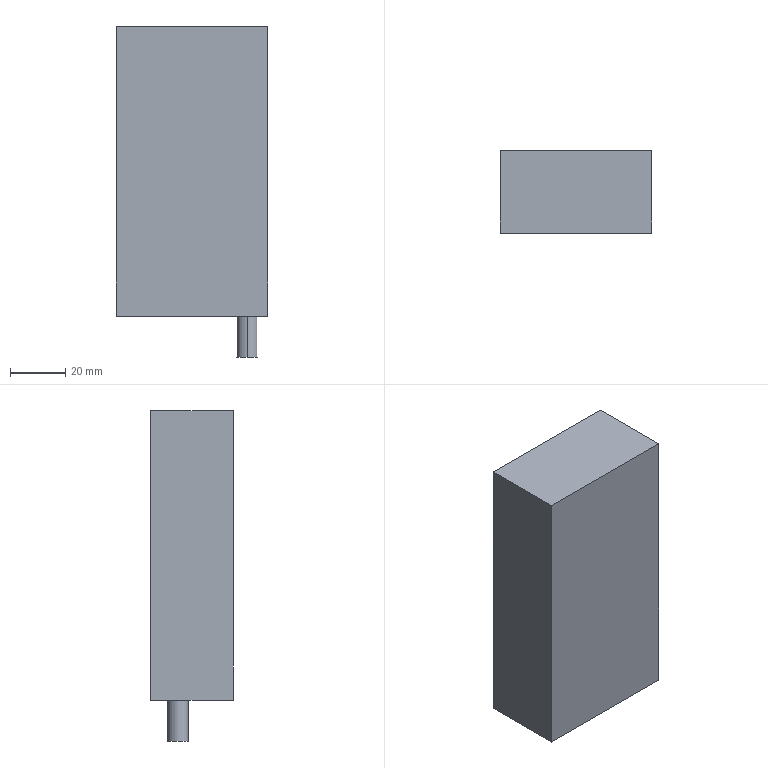Part | SolidWorks | features BaseBody 1 | 1 solid | 33 faces | box 55 x 30 x 120 mm | volume 172847 mm3 | cylinder 14 | cone 12 | plane 7 | commonest cylinder face diameters 4.2 x12 7.5 x2
STEP:
#1=CARTESIAN_POINT('',(47.5,23.75,-15.));
#2=VERTEX_POINT('',#1);
#3=CARTESIAN_POINT('',(47.5,16.25,-15.));
#4=VERTEX_POINT('',#3);
#5=CARTESIAN_POINT('',(47.5,20.,-15.));
#6=DIRECTION('',(0.,0.,-1.));
#7=DIRECTION('',(0.,-1.,0.));
#8=AXIS2_PLACEMENT_3D('',#5,#6,#7);
#9=CIRCLE('',#8,3.75);
#10=EDGE_CURVE('',#2,#4,#9,.T.);
#11=ORIENTED_EDGE('',*,*,#10,.F.);
#12=CARTESIAN_POINT('',(47.5,23.75,0.));
#13=VERTEX_POINT('',#12);
#14=CARTESIAN_POINT('',(47.5,23.75,-15.));
#15=DIRECTION('',(0.,0.,1.));
#16=VECTOR('',#15,1000.);
#17=LINE('',#14,#16);
#18=EDGE_CURVE('',#2,#13,#17,.T.);
#19=ORIENTED_EDGE('',*,*,#18,.T.);
#20=CARTESIAN_POINT('',(47.5,16.25,0.));
#21=VERTEX_POINT('',#20);
#22=CARTESIAN_POINT('',(47.5,20.,0.));
#23=DIRECTION('',(0.,0.,1.));
#24=DIRECTION('',(0.,-1.,0.));
#25=AXIS2_PLACEMENT_3D('',#22,#23,#24);
#26=CIRCLE('',#25,3.75);
#27=EDGE_CURVE('',#21,#13,#26,.T.);
#28=ORIENTED_EDGE('',*,*,#27,.F.);
#29=CARTESIAN_POINT('',(47.5,16.25,-15.));
#30=DIRECTION('',(0.,0.,1.));
#31=VECTOR('',#30,1000.);
#32=LINE('',#29,#31);
#33=EDGE_CURVE('',#4,#21,#32,.T.);
#34=ORIENTED_EDGE('',*,*,#33,.F.);
#35=EDGE_LOOP('',(#11,#19,#28,#34));
#36=FACE_OUTER_BOUND('',#35,.T.);
#37=CARTESIAN_POINT('',(47.5,20.,-15.));
#38=DIRECTION('',(0.,0.,1.));
#39=DIRECTION('',(0.,-1.,0.));
#40=AXIS2_PLACEMENT_3D('',#37,#38,#39);
#41=CYLINDRICAL_SURFACE('',#40,3.75);
#42=ADVANCED_FACE('',(#36),#41,.T.);
#43=CARTESIAN_POINT('',(50.,17.6,17.1));
#44=VERTEX_POINT('',#43);
#45=CARTESIAN_POINT('',(50.,17.6,12.9));
#46=VERTEX_POINT('',#45);
#47=CARTESIAN_POINT('',(50.,17.6,15.));
#48=DIRECTION('',(0.,-1.,0.));
#49=DIRECTION('',(0.,0.,1.));
#50=AXIS2_PLACEMENT_3D('',#47,#48,#49);
#51=CIRCLE('',#50,2.1);
#52=EDGE_CURVE('',#44,#46,#51,.T.);
#53=ORIENTED_EDGE('',*,*,#52,.T.);
#54=CARTESIAN_POINT('',(50.,30.,12.9));
#55=VERTEX_POINT('',#54);
#56=CARTESIAN_POINT('',(50.,17.6,12.9));
#57=DIRECTION('',(0.,1.,0.));
#58=VECTOR('',#57,1000.);
#59=LINE('',#56,#58);
#60=EDGE_CURVE('',#46,#55,#59,.T.);
#61=ORIENTED_EDGE('',*,*,#60,.T.);
#62=CARTESIAN_POINT('',(50.,30.,17.1));
#63=VERTEX_POINT('',#62);
#64=CARTESIAN_POINT('',(50.,30.,15.));
#65=DIRECTION('',(0.,1.,0.));
#66=DIRECTION('',(0.,0.,1.));
#67=AXIS2_PLACEMENT_3D('',#64,#65,#66);
#68=CIRCLE('',#67,2.1);
#69=EDGE_CURVE('',#55,#63,#68,.T.);
#70=ORIENTED_EDGE('',*,*,#69,.T.);
#71=CARTESIAN_POINT('',(50.,17.6,17.1));
#72=DIRECTION('',(0.,1.,0.));
#73=VECTOR('',#72,1000.);
#74=LINE('',#71,#73);
#75=EDGE_CURVE('',#44,#63,#74,.T.);
#76=ORIENTED_EDGE('',*,*,#75,.F.);
#77=EDGE_LOOP('',(#53,#61,#70,#76));
#78=FACE_OUTER_BOUND('',#77,.T.);
#79=CARTESIAN_POINT('',(50.,17.6,15.));
#80=DIRECTION('',(0.,1.,0.));
#81=DIRECTION('',(0.,0.,1.));
#82=AXIS2_PLACEMENT_3D('',#79,#80,#81);
#83=CYLINDRICAL_SURFACE('',#82,2.1);
#84=ADVANCED_FACE('',(#78),#83,.F.);
#85=CARTESIAN_POINT('',(5.,17.6,17.1));
#86=VERTEX_POINT('',#85);
#87=CARTESIAN_POINT('',(5.,17.6,12.9));
#88=VERTEX_POINT('',#87);
#89=CARTESIAN_POINT('',(5.,17.6,15.));
#90=DIRECTION('',(0.,-1.,0.));
#91=DIRECTION('',(0.,0.,1.));
#92=AXIS2_PLACEMENT_3D('',#89,#90,#91);
#93=CIRCLE('',#92,2.1);
#94=EDGE_CURVE('',#86,#88,#93,.T.);
#95=ORIENTED_EDGE('',*,*,#94,.T.);
#96=CARTESIAN_POINT('',(5.,30.,12.9));
#97=VERTEX_POINT('',#96);
#98=CARTESIAN_POINT('',(5.,17.6,12.9));
#99=DIRECTION('',(0.,1.,0.));
#100=VECTOR('',#99,1000.);
#101=LINE('',#98,#100);
#102=EDGE_CURVE('',#88,#97,#101,.T.);
#103=ORIENTED_EDGE('',*,*,#102,.T.);
#104=CARTESIAN_POINT('',(5.,30.,17.1));
#105=VERTEX_POINT('',#104);
#106=CARTESIAN_POINT('',(5.,30.,15.));
#107=DIRECTION('',(0.,1.,0.));
#108=DIRECTION('',(0.,0.,1.));
#109=AXIS2_PLACEMENT_3D('',#106,#107,#108);
#110=CIRCLE('',#109,2.1);
#111=EDGE_CURVE('',#97,#105,#110,.T.);
#112=ORIENTED_EDGE('',*,*,#111,.T.);
#113=CARTESIAN_POINT('',(5.,17.6,17.1));
#114=DIRECTION('',(0.,1.,0.));
#115=VECTOR('',#114,1000.);
#116=LINE('',#113,#115);
#117=EDGE_CURVE('',#86,#105,#116,.T.);
#118=ORIENTED_EDGE('',*,*,#117,.F.);
#119=EDGE_LOOP('',(#95,#103,#112,#118));
#120=FACE_OUTER_BOUND('',#119,.T.);
#121=CARTESIAN_POINT('',(5.,17.6,15.));
#122=DIRECTION('',(0.,1.,0.));
#123=DIRECTION('',(0.,0.,1.));
#124=AXIS2_PLACEMENT_3D('',#121,#122,#123);
#125=CYLINDRICAL_SURFACE('',#124,2.1);
#126=ADVANCED_FACE('',(#120),#125,.F.);
#127=CARTESIAN_POINT('',(50.,17.6,54.6));
#128=VERTEX_POINT('',#127);
#129=CARTESIAN_POINT('',(50.,17.6,50.4));
#130=VERTEX_POINT('',#129);
#131=CARTESIAN_POINT('',(50.,17.6,52.5));
#132=DIRECTION('',(0.,-1.,0.));
#133=DIRECTION('',(0.,0.,1.));
#134=AXIS2_PLACEMENT_3D('',#131,#132,#133);
#135=CIRCLE('',#134,2.1);
#136=EDGE_CURVE('',#128,#130,#135,.T.);
#137=ORIENTED_EDGE('',*,*,#136,.T.);
#138=CARTESIAN_POINT('',(50.,30.,50.4));
#139=VERTEX_POINT('',#138);
#140=CARTESIAN_POINT('',(50.,17.6,50.4));
#141=DIRECTION('',(0.,1.,0.));
#142=VECTOR('',#141,1000.);
#143=LINE('',#140,#142);
#144=EDGE_CURVE('',#130,#139,#143,.T.);
#145=ORIENTED_EDGE('',*,*,#144,.T.);
#146=CARTESIAN_POINT('',(50.,30.,54.6));
#147=VERTEX_POINT('',#146);
#148=CARTESIAN_POINT('',(50.,30.,52.5));
#149=DIRECTION('',(0.,1.,0.));
#150=DIRECTION('',(0.,0.,1.));
#151=AXIS2_PLACEMENT_3D('',#148,#149,#150);
#152=CIRCLE('',#151,2.1);
#153=EDGE_CURVE('',#139,#147,#152,.T.);
#154=ORIENTED_EDGE('',*,*,#153,.T.);
#155=CARTESIAN_POINT('',(50.,17.6,54.6));
#156=DIRECTION('',(0.,1.,0.));
#157=VECTOR('',#156,1000.);
#158=LINE('',#155,#157);
#159=EDGE_CURVE('',#128,#147,#158,.T.);
#160=ORIENTED_EDGE('',*,*,#159,.F.);
#161=EDGE_LOOP('',(#137,#145,#154,#160));
#162=FACE_OUTER_BOUND('',#161,.T.);
#163=CARTESIAN_POINT('',(50.,17.6,52.5));
#164=DIRECTION('',(0.,1.,0.));
#165=DIRECTION('',(0.,0.,1.));
#166=AXIS2_PLACEMENT_3D('',#163,#164,#165);
#167=CYLINDRICAL_SURFACE('',#166,2.1);
#168=ADVANCED_FACE('',(#162),#167,.F.);
#169=CARTESIAN_POINT('',(5.,17.6,54.6));
#170=VERTEX_POINT('',#169);
#171=CARTESIAN_POINT('',(5.,17.6,50.4));
#172=VERTEX_POINT('',#171);
#173=CARTESIAN_POINT('',(5.,17.6,52.5));
#174=DIRECTION('',(0.,-1.,0.));
#175=DIRECTION('',(0.,0.,1.));
#176=AXIS2_PLACEMENT_3D('',#173,#174,#175);
#177=CIRCLE('',#176,2.1);
#178=EDGE_CURVE('',#170,#172,#177,.T.);
#179=ORIENTED_EDGE('',*,*,#178,.T.);
#180=CARTESIAN_POINT('',(5.,30.,50.4));
#181=VERTEX_POINT('',#180);
#182=CARTESIAN_POINT('',(5.,17.6,50.4));
#183=DIRECTION('',(0.,1.,0.));
#184=VECTOR('',#183,1000.);
#185=LINE('',#182,#184);
#186=EDGE_CURVE('',#172,#181,#185,.T.);
#187=ORIENTED_EDGE('',*,*,#186,.T.);
#188=CARTESIAN_POINT('',(5.,30.,54.6));
#189=VERTEX_POINT('',#188);
#190=CARTESIAN_POINT('',(5.,30.,52.5));
#191=DIRECTION('',(0.,1.,0.));
#192=DIRECTION('',(0.,0.,1.));
#193=AXIS2_PLACEMENT_3D('',#190,#191,#192);
#194=CIRCLE('',#193,2.1);
#195=EDGE_CURVE('',#181,#189,#194,.T.);
#196=ORIENTED_EDGE('',*,*,#195,.T.);
#197=CARTESIAN_POINT('',(5.,17.6,54.6));
#198=DIRECTION('',(0.,1.,0.));
#199=VECTOR('',#198,1000.);
#200=LINE('',#197,#199);
#201=EDGE_CURVE('',#170,#189,#200,.T.);
#202=ORIENTED_EDGE('',*,*,#201,.F.);
#203=EDGE_LOOP('',(#179,#187,#196,#202));
#204=FACE_OUTER_BOUND('',#203,.T.);
#205=CARTESIAN_POINT('',(5.,17.6,52.5));
#206=DIRECTION('',(0.,1.,0.));
#207=DIRECTION('',(0.,0.,1.));
#208=AXIS2_PLACEMENT_3D('',#205,#206,#207);
#209=CYLINDRICAL_SURFACE('',#208,2.1);
#210=ADVANCED_FACE('',(#204),#209,.F.);
#211=CARTESIAN_POINT('',(50.,17.6,92.1));
#212=VERTEX_POINT('',#211);
#213=CARTESIAN_POINT('',(50.,17.6,87.9));
#214=VERTEX_POINT('',#213);
#215=CARTESIAN_POINT('',(50.,17.6,90.));
#216=DIRECTION('',(0.,-1.,0.));
#217=DIRECTION('',(0.,0.,1.));
#218=AXIS2_PLACEMENT_3D('',#215,#216,#217);
#219=CIRCLE('',#218,2.1);
#220=EDGE_CURVE('',#212,#214,#219,.T.);
#221=ORIENTED_EDGE('',*,*,#220,.T.);
#222=CARTESIAN_POINT('',(50.,30.,87.9));
#223=VERTEX_POINT('',#222);
#224=CARTESIAN_POINT('',(50.,17.6,87.9));
#225=DIRECTION('',(0.,1.,0.));
#226=VECTOR('',#225,1000.);
#227=LINE('',#224,#226);
#228=EDGE_CURVE('',#214,#223,#227,.T.);
#229=ORIENTED_EDGE('',*,*,#228,.T.);
#230=CARTESIAN_POINT('',(50.,30.,92.1));
#231=VERTEX_POINT('',#230);
#232=CARTESIAN_POINT('',(50.,30.,90.));
#233=DIRECTION('',(0.,1.,0.));
#234=DIRECTION('',(0.,0.,1.));
#235=AXIS2_PLACEMENT_3D('',#232,#233,#234);
#236=CIRCLE('',#235,2.1);
#237=EDGE_CURVE('',#223,#231,#236,.T.);
#238=ORIENTED_EDGE('',*,*,#237,.T.);
#239=CARTESIAN_POINT('',(50.,17.6,92.1));
#240=DIRECTION('',(0.,1.,0.));
#241=VECTOR('',#240,1000.);
#242=LINE('',#239,#241);
#243=EDGE_CURVE('',#212,#231,#242,.T.);
#244=ORIENTED_EDGE('',*,*,#243,.F.);
#245=EDGE_LOOP('',(#221,#229,#238,#244));
#246=FACE_OUTER_BOUND('',#245,.T.);
#247=CARTESIAN_POINT('',(50.,17.6,90.));
#248=DIRECTION('',(0.,1.,0.));
#249=DIRECTION('',(0.,0.,1.));
#250=AXIS2_PLACEMENT_3D('',#247,#248,#249);
#251=CYLINDRICAL_SURFACE('',#250,2.1);
#252=ADVANCED_FACE('',(#246),#251,.F.);
#253=CARTESIAN_POINT('',(5.,17.6,92.1));
#254=VERTEX_POINT('',#253);
#255=CARTESIAN_POINT('',(5.,17.6,87.9));
#256=VERTEX_POINT('',#255);
#257=CARTESIAN_POINT('',(5.,17.6,90.));
#258=DIRECTION('',(0.,-1.,0.));
#259=DIRECTION('',(0.,0.,1.));
#260=AXIS2_PLACEMENT_3D('',#257,#258,#259);
#261=CIRCLE('',#260,2.1);
#262=EDGE_CURVE('',#254,#256,#261,.T.);
#263=ORIENTED_EDGE('',*,*,#262,.T.);
#264=CARTESIAN_POINT('',(5.,30.,87.9));
#265=VERTEX_POINT('',#264);
#266=CARTESIAN_POINT('',(5.,17.6,87.9));
#267=DIRECTION('',(0.,1.,0.));
#268=VECTOR('',#267,1000.);
#269=LINE('',#266,#268);
#270=EDGE_CURVE('',#256,#265,#269,.T.);
#271=ORIENTED_EDGE('',*,*,#270,.T.);
#272=CARTESIAN_POINT('',(5.,30.,92.1));
#273=VERTEX_POINT('',#272);
#274=CARTESIAN_POINT('',(5.,30.,90.));
#275=DIRECTION('',(0.,1.,0.));
#276=DIRECTION('',(0.,0.,1.));
#277=AXIS2_PLACEMENT_3D('',#274,#275,#276);
#278=CIRCLE('',#277,2.1);
#279=EDGE_CURVE('',#265,#273,#278,.T.);
#280=ORIENTED_EDGE('',*,*,#279,.T.);
#281=CARTESIAN_POINT('',(5.,17.6,92.1));
#282=DIRECTION('',(0.,1.,0.));
#283=VECTOR('',#282,1000.);
#284=LINE('',#281,#283);
#285=EDGE_CURVE('',#254,#273,#284,.T.);
#286=ORIENTED_EDGE('',*,*,#285,.F.);
#287=EDGE_LOOP('',(#263,#271,#280,#286));
#288=FACE_OUTER_BOUND('',#287,.T.);
#289=CARTESIAN_POINT('',(5.,17.6,90.));
#290=DIRECTION('',(0.,1.,0.));
#291=DIRECTION('',(0.,0.,1.));
#292=AXIS2_PLACEMENT_3D('',#289,#290,#291);
#293=CYLINDRICAL_SURFACE('',#292,2.1);
#294=ADVANCED_FACE('',(#288),#293,.F.);
#295=CARTESIAN_POINT('',(50.,16.338,15.));
#296=VERTEX_POINT('',#295);
#297=CARTESIAN_POINT('',(50.,16.338,15.));
#298=DIRECTION('',(0.,0.515,0.8572));
#299=VECTOR('',#298,1000.);
#300=LINE('',#297,#299);
#301=EDGE_CURVE('',#296,#44,#300,.T.);
#302=ORIENTED_EDGE('',*,*,#301,.F.);
#303=CARTESIAN_POINT('',(50.,16.338,15.));
#304=DIRECTION('',(0.,0.515,-0.8572));
#305=VECTOR('',#304,1000.);
#306=LINE('',#303,#305);
#307=EDGE_CURVE('',#296,#46,#306,.T.);
#308=ORIENTED_EDGE('',*,*,#307,.T.);
#309=ORIENTED_EDGE('',*,*,#52,.F.);
#310=EDGE_LOOP('',(#302,#308,#309));
#311=FACE_OUTER_BOUND('',#310,.T.);
#312=CARTESIAN_POINT('',(50.,1016.338,15.));
#313=DIRECTION('',(0.,1.,0.));
#314=DIRECTION('',(0.,0.,1.));
#315=AXIS2_PLACEMENT_3D('',#312,#313,#314);
#316=CONICAL_SURFACE('',#315,1664.279,1.03);
#317=ADVANCED_FACE('',(#311),#316,.F.);
#318=CARTESIAN_POINT('',(5.,16.338,15.));
#319=VERTEX_POINT('',#318);
#320=CARTESIAN_POINT('',(5.,16.338,15.));
#321=DIRECTION('',(0.,0.515,0.8572));
#322=VECTOR('',#321,1000.);
#323=LINE('',#320,#322);
#324=EDGE_CURVE('',#319,#86,#323,.T.);
#325=ORIENTED_EDGE('',*,*,#324,.F.);
#326=CARTESIAN_POINT('',(5.,16.338,15.));
#327=DIRECTION('',(0.,0.515,-0.8572));
#328=VECTOR('',#327,1000.);
#329=LINE('',#326,#328);
#330=EDGE_CURVE('',#319,#88,#329,.T.);
#331=ORIENTED_EDGE('',*,*,#330,.T.);
#332=ORIENTED_EDGE('',*,*,#94,.F.);
#333=EDGE_LOOP('',(#325,#331,#332));
#334=FACE_OUTER_BOUND('',#333,.T.);
#335=CARTESIAN_POINT('',(5.,1016.338,15.));
#336=DIRECTION('',(0.,1.,0.));
#337=DIRECTION('',(0.,0.,1.));
#338=AXIS2_PLACEMENT_3D('',#335,#336,#337);
#339=CONICAL_SURFACE('',#338,1664.279,1.03);
#340=ADVANCED_FACE('',(#334),#339,.F.);
#341=CARTESIAN_POINT('',(50.,16.338,52.5));
#342=VERTEX_POINT('',#341);
#343=CARTESIAN_POINT('',(50.,16.338,52.5));
#344=DIRECTION('',(0.,0.515,0.8572));
#345=VECTOR('',#344,1000.);
#346=LINE('',#343,#345);
#347=EDGE_CURVE('',#342,#128,#346,.T.);
#348=ORIENTED_EDGE('',*,*,#347,.F.);
#349=CARTESIAN_POINT('',(50.,16.338,52.5));
#350=DIRECTION('',(0.,0.515,-0.8572));
#351=VECTOR('',#350,1000.);
#352=LINE('',#349,#351);
#353=EDGE_CURVE('',#342,#130,#352,.T.);
#354=ORIENTED_EDGE('',*,*,#353,.T.);
#355=ORIENTED_EDGE('',*,*,#136,.F.);
#356=EDGE_LOOP('',(#348,#354,#355));
#357=FACE_OUTER_BOUND('',#356,.T.);
#358=CARTESIAN_POINT('',(50.,1016.338,52.5));
#359=DIRECTION('',(0.,1.,0.));
#360=DIRECTION('',(0.,0.,1.));
#361=AXIS2_PLACEMENT_3D('',#358,#359,#360);
#362=CONICAL_SURFACE('',#361,1664.279,1.03);
#363=ADVANCED_FACE('',(#357),#362,.F.);
#364=CARTESIAN_POINT('',(5.,16.338,52.5));
#365=VERTEX_POINT('',#364);
#366=CARTESIAN_POINT('',(5.,16.338,52.5));
#367=DIRECTION('',(0.,0.515,0.8572));
#368=VECTOR('',#367,1000.);
#369=LINE('',#366,#368);
#370=EDGE_CURVE('',#365,#170,#369,.T.);
#371=ORIENTED_EDGE('',*,*,#370,.F.);
#372=CARTESIAN_POINT('',(5.,16.338,52.5));
#373=DIRECTION('',(0.,0.515,-0.8572));
#374=VECTOR('',#373,1000.);
#375=LINE('',#372,#374);
#376=EDGE_CURVE('',#365,#172,#375,.T.);
#377=ORIENTED_EDGE('',*,*,#376,.T.);
#378=ORIENTED_EDGE('',*,*,#178,.F.);
#379=EDGE_LOOP('',(#371,#377,#378));
#380=FACE_OUTER_BOUND('',#379,.T.);
#381=CARTESIAN_POINT('',(5.,1016.338,52.5));
#382=DIRECTION('',(0.,1.,0.));
#383=DIRECTION('',(0.,0.,1.));
#384=AXIS2_PLACEMENT_3D('',#381,#382,#383);
#385=CONICAL_SURFACE('',#384,1664.279,1.03);
#386=ADVANCED_FACE('',(#380),#385,.F.);
#387=CARTESIAN_POINT('',(50.,16.338,90.));
#388=VERTEX_POINT('',#387);
#389=CARTESIAN_POINT('',(50.,16.338,90.));
#390=DIRECTION('',(0.,0.515,0.8572));
#391=VECTOR('',#390,1000.);
#392=LINE('',#389,#391);
#393=EDGE_CURVE('',#388,#212,#392,.T.);
#394=ORIENTED_EDGE('',*,*,#393,.F.);
#395=CARTESIAN_POINT('',(50.,16.338,90.));
#396=DIRECTION('',(0.,0.515,-0.8572));
#397=VECTOR('',#396,1000.);
#398=LINE('',#395,#397);
#399=EDGE_CURVE('',#388,#214,#398,.T.);
#400=ORIENTED_EDGE('',*,*,#399,.T.);
#401=ORIENTED_EDGE('',*,*,#220,.F.);
#402=EDGE_LOOP('',(#394,#400,#401));
#403=FACE_OUTER_BOUND('',#402,.T.);
#404=CARTESIAN_POINT('',(50.,1016.338,90.));
#405=DIRECTION('',(0.,1.,0.));
#406=DIRECTION('',(0.,0.,1.));
#407=AXIS2_PLACEMENT_3D('',#404,#405,#406);
#408=CONICAL_SURFACE('',#407,1664.279,1.03);
#409=ADVANCED_FACE('',(#403),#408,.F.);
#410=CARTESIAN_POINT('',(5.,16.338,90.));
#411=VERTEX_POINT('',#410);
#412=CARTESIAN_POINT('',(5.,16.338,90.));
#413=DIRECTION('',(0.,0.515,0.8572));
#414=VECTOR('',#413,1000.);
#415=LINE('',#412,#414);
#416=EDGE_CURVE('',#411,#254,#415,.T.);
#417=ORIENTED_EDGE('',*,*,#416,.F.);
#418=CARTESIAN_POINT('',(5.,16.338,90.));
#419=DIRECTION('',(0.,0.515,-0.8572));
#420=VECTOR('',#419,1000.);
#421=LINE('',#418,#420);
#422=EDGE_CURVE('',#411,#256,#421,.T.);
#423=ORIENTED_EDGE('',*,*,#422,.T.);
#424=ORIENTED_EDGE('',*,*,#262,.F.);
#425=EDGE_LOOP('',(#417,#423,#424));
#426=FACE_OUTER_BOUND('',#425,.T.);
#427=CARTESIAN_POINT('',(5.,1016.338,90.));
#428=DIRECTION('',(0.,1.,0.));
#429=DIRECTION('',(0.,0.,1.));
#430=AXIS2_PLACEMENT_3D('',#427,#428,#429);
#431=CONICAL_SURFACE('',#430,1664.279,1.03);
#432=ADVANCED_FACE('',(#426),#431,.F.);
#433=ORIENTED_EDGE('',*,*,#18,.F.);
#434=CARTESIAN_POINT('',(47.5,20.,-15.));
#435=DIRECTION('',(0.,0.,-1.));
#436=DIRECTION('',(0.,-1.,0.));
#437=AXIS2_PLACEMENT_3D('',#434,#435,#436);
#438=CIRCLE('',#437,3.75);
#439=EDGE_CURVE('',#4,#2,#438,.T.);
#440=ORIENTED_EDGE('',*,*,#439,.F.);
#441=ORIENTED_EDGE('',*,*,#33,.T.);
#442=CARTESIAN_POINT('',(47.5,20.,0.));
#443=DIRECTION('',(0.,0.,1.));
#444=DIRECTION('',(0.,-1.,0.));
#445=AXIS2_PLACEMENT_3D('',#442,#443,#444);
#446=CIRCLE('',#445,3.75);
#447=EDGE_CURVE('',#13,#21,#446,.T.);
#448=ORIENTED_EDGE('',*,*,#447,.F.);
#449=EDGE_LOOP('',(#433,#440,#441,#448));
#450=FACE_OUTER_BOUND('',#449,.T.);
#451=CARTESIAN_POINT('',(47.5,20.,-15.));
#452=DIRECTION('',(0.,0.,1.));
#453=DIRECTION('',(0.,-1.,0.));
#454=AXIS2_PLACEMENT_3D('',#451,#452,#453);
#455=CYLINDRICAL_SURFACE('',#454,3.75);
#456=ADVANCED_FACE('',(#450),#455,.T.);
#457=ORIENTED_EDGE('',*,*,#439,.T.);
#458=ORIENTED_EDGE('',*,*,#10,.T.);
#459=EDGE_LOOP('',(#457,#458));
#460=FACE_OUTER_BOUND('',#459,.T.);
#461=CARTESIAN_POINT('',(51.295,16.205,-15.));
#462=DIRECTION('',(0.,0.,-1.));
#463=DIRECTION('',(-1.,0.,0.));
#464=AXIS2_PLACEMENT_3D('',#461,#462,#463);
#465=PLANE('',#464);
#466=ADVANCED_FACE('',(#460),#465,.T.);
#467=ORIENTED_EDGE('',*,*,#27,.T.);
#468=ORIENTED_EDGE('',*,*,#447,.T.);
#469=EDGE_LOOP('',(#467,#468));
#470=FACE_BOUND('',#469,.T.);
#471=CARTESIAN_POINT('',(0.,0.,0.));
#472=VERTEX_POINT('',#471);
#473=CARTESIAN_POINT('',(0.,30.,0.));
#474=VERTEX_POINT('',#473);
#475=CARTESIAN_POINT('',(0.,15.,0.));
#476=DIRECTION('',(0.,1.,0.));
#477=VECTOR('',#476,1000.);
#478=LINE('',#475,#477);
#479=EDGE_CURVE('',#472,#474,#478,.T.);
#480=ORIENTED_EDGE('',*,*,#479,.T.);
#481=CARTESIAN_POINT('',(55.,30.,0.));
#482=VERTEX_POINT('',#481);
#483=CARTESIAN_POINT('',(27.5,30.,0.));
#484=DIRECTION('',(1.,0.,0.));
#485=VECTOR('',#484,1000.);
#486=LINE('',#483,#485);
#487=EDGE_CURVE('',#474,#482,#486,.T.);
#488=ORIENTED_EDGE('',*,*,#487,.T.);
#489=CARTESIAN_POINT('',(55.,0.,0.));
#490=VERTEX_POINT('',#489);
#491=CARTESIAN_POINT('',(55.,15.,0.));
#492=DIRECTION('',(0.,-1.,0.));
#493=VECTOR('',#492,1000.);
#494=LINE('',#491,#493);
#495=EDGE_CURVE('',#482,#490,#494,.T.);
#496=ORIENTED_EDGE('',*,*,#495,.T.);
#497=CARTESIAN_POINT('',(27.5,0.,0.));
#498=DIRECTION('',(-1.,0.,0.));
#499=VECTOR('',#498,1000.);
#500=LINE('',#497,#499);
#501=EDGE_CURVE('',#490,#472,#500,.T.);
#502=ORIENTED_EDGE('',*,*,#501,.T.);
#503=EDGE_LOOP('',(#480,#488,#496,#502));
#504=FACE_OUTER_BOUND('',#503,.T.);
#505=CARTESIAN_POINT('',(55.,0.,0.));
#506=DIRECTION('',(0.,0.,-1.));
#507=DIRECTION('',(-1.,0.,0.));
#508=AXIS2_PLACEMENT_3D('',#505,#506,#507);
#509=PLANE('',#508);
#510=ADVANCED_FACE('',(#470,#504),#509,.T.);
#511=CARTESIAN_POINT('',(50.,30.,15.));
#512=DIRECTION('',(0.,1.,0.));
#513=DIRECTION('',(0.,0.,1.));
#514=AXIS2_PLACEMENT_3D('',#511,#512,#513);
#515=CIRCLE('',#514,2.1);
#516=EDGE_CURVE('',#63,#55,#515,.T.);
#517=ORIENTED_EDGE('',*,*,#516,.F.);
#518=ORIENTED_EDGE('',*,*,#69,.F.);
#519=EDGE_LOOP('',(#517,#518));
#520=FACE_BOUND('',#519,.T.);
#521=CARTESIAN_POINT('',(5.,30.,15.));
#522=DIRECTION('',(0.,1.,0.));
#523=DIRECTION('',(0.,0.,1.));
#524=AXIS2_PLACEMENT_3D('',#521,#522,#523);
#525=CIRCLE('',#524,2.1);
#526=EDGE_CURVE('',#105,#97,#525,.T.);
#527=ORIENTED_EDGE('',*,*,#526,.F.);
#528=ORIENTED_EDGE('',*,*,#111,.F.);
#529=EDGE_LOOP('',(#527,#528));
#530=FACE_BOUND('',#529,.T.);
#531=CARTESIAN_POINT('',(50.,30.,52.5));
#532=DIRECTION('',(0.,1.,0.));
#533=DIRECTION('',(0.,0.,1.));
#534=AXIS2_PLACEMENT_3D('',#531,#532,#533);
#535=CIRCLE('',#534,2.1);
#536=EDGE_CURVE('',#147,#139,#535,.T.);
#537=ORIENTED_EDGE('',*,*,#536,.F.);
#538=ORIENTED_EDGE('',*,*,#153,.F.);
#539=EDGE_LOOP('',(#537,#538));
#540=FACE_BOUND('',#539,.T.);
#541=CARTESIAN_POINT('',(5.,30.,52.5));
#542=DIRECTION('',(0.,1.,0.));
#543=DIRECTION('',(0.,0.,1.));
#544=AXIS2_PLACEMENT_3D('',#541,#542,#543);
#545=CIRCLE('',#544,2.1);
#546=EDGE_CURVE('',#189,#181,#545,.T.);
#547=ORIENTED_EDGE('',*,*,#546,.F.);
#548=ORIENTED_EDGE('',*,*,#195,.F.);
#549=EDGE_LOOP('',(#547,#548));
#550=FACE_BOUND('',#549,.T.);
#551=CARTESIAN_POINT('',(50.,30.,90.));
#552=DIRECTION('',(0.,1.,0.));
#553=DIRECTION('',(0.,0.,1.));
#554=AXIS2_PLACEMENT_3D('',#551,#552,#553);
#555=CIRCLE('',#554,2.1);
#556=EDGE_CURVE('',#231,#223,#555,.T.);
#557=ORIENTED_EDGE('',*,*,#556,.F.);
#558=ORIENTED_EDGE('',*,*,#237,.F.);
#559=EDGE_LOOP('',(#557,#558));
#560=FACE_BOUND('',#559,.T.);
#561=CARTESIAN_POINT('',(5.,30.,90.));
#562=DIRECTION('',(0.,1.,0.));
#563=DIRECTION('',(0.,0.,1.));
#564=AXIS2_PLACEMENT_3D('',#561,#562,#563);
#565=CIRCLE('',#564,2.1);
#566=EDGE_CURVE('',#273,#265,#565,.T.);
#567=ORIENTED_EDGE('',*,*,#566,.F.);
#568=ORIENTED_EDGE('',*,*,#279,.F.);
#569=EDGE_LOOP('',(#567,#568));
#570=FACE_BOUND('',#569,.T.);
#571=CARTESIAN_POINT('',(55.,30.,105.));
#572=VERTEX_POINT('',#571);
#573=CARTESIAN_POINT('',(0.,30.,105.));
#574=VERTEX_POINT('',#573);
#575=CARTESIAN_POINT('',(27.5,30.,105.));
#576=DIRECTION('',(-1.,0.,0.));
#577=VECTOR('',#576,1000.);
#578=LINE('',#575,#577);
#579=EDGE_CURVE('',#572,#574,#578,.T.);
#580=ORIENTED_EDGE('',*,*,#579,.F.);
#581=CARTESIAN_POINT('',(55.,30.,52.5));
#582=DIRECTION('',(0.,0.,1.));
#583=VECTOR('',#582,1000.);
#584=LINE('',#581,#583);
#585=EDGE_CURVE('',#482,#572,#584,.T.);
#586=ORIENTED_EDGE('',*,*,#585,.F.);
#587=ORIENTED_EDGE('',*,*,#487,.F.);
#588=CARTESIAN_POINT('',(0.,30.,52.5));
#589=DIRECTION('',(0.,0.,-1.));
#590=VECTOR('',#589,1000.);
#591=LINE('',#588,#590);
#592=EDGE_CURVE('',#574,#474,#591,.T.);
#593=ORIENTED_EDGE('',*,*,#592,.F.);
#594=EDGE_LOOP('',(#580,#586,#587,#593));
#595=FACE_OUTER_BOUND('',#594,.T.);
#596=CARTESIAN_POINT('',(0.,30.,105.));
#597=DIRECTION('',(0.,-1.,0.));
#598=DIRECTION('',(0.,0.,-1.));
#599=AXIS2_PLACEMENT_3D('',#596,#597,#598);
#600=PLANE('',#599);
#601=ADVANCED_FACE('',(#520,#530,#540,#550,#560,#570,#595),#600,.F.);
#602=CARTESIAN_POINT('',(0.,0.,105.));
#603=VERTEX_POINT('',#602);
#604=CARTESIAN_POINT('',(0.,15.,105.));
#605=DIRECTION('',(0.,-1.,0.));
#606=VECTOR('',#605,1000.);
#607=LINE('',#604,#606);
#608=EDGE_CURVE('',#574,#603,#607,.T.);
#609=ORIENTED_EDGE('',*,*,#608,.F.);
#610=ORIENTED_EDGE('',*,*,#592,.T.);
#611=ORIENTED_EDGE('',*,*,#479,.F.);
#612=CARTESIAN_POINT('',(0.,0.,52.5));
#613=DIRECTION('',(0.,0.,-1.));
#614=VECTOR('',#613,1000.);
#615=LINE('',#612,#614);
#616=EDGE_CURVE('',#603,#472,#615,.T.);
#617=ORIENTED_EDGE('',*,*,#616,.F.);
#618=EDGE_LOOP('',(#609,#610,#611,#617));
#619=FACE_OUTER_BOUND('',#618,.T.);
#620=CARTESIAN_POINT('',(0.,0.,105.));
#621=DIRECTION('',(1.,0.,0.));
#622=DIRECTION('',(0.,0.,-1.));
#623=AXIS2_PLACEMENT_3D('',#620,#621,#622);
#624=PLANE('',#623);
#625=ADVANCED_FACE('',(#619),#624,.F.);
#626=CARTESIAN_POINT('',(55.,0.,105.));
#627=VERTEX_POINT('',#626);
#628=CARTESIAN_POINT('',(27.5,0.,105.));
#629=DIRECTION('',(1.,0.,0.));
#630=VECTOR('',#629,1000.);
#631=LINE('',#628,#630);
#632=EDGE_CURVE('',#603,#627,#631,.T.);
#633=ORIENTED_EDGE('',*,*,#632,.F.);
#634=ORIENTED_EDGE('',*,*,#616,.T.);
#635=ORIENTED_EDGE('',*,*,#501,.F.);
#636=CARTESIAN_POINT('',(55.,0.,52.5));
#637=DIRECTION('',(0.,0.,-1.));
#638=VECTOR('',#637,1000.);
#639=LINE('',#636,#638);
#640=EDGE_CURVE('',#627,#490,#639,.T.);
#641=ORIENTED_EDGE('',*,*,#640,.F.);
#642=EDGE_LOOP('',(#633,#634,#635,#641));
#643=FACE_OUTER_BOUND('',#642,.T.);
#644=CARTESIAN_POINT('',(0.,0.,0.));
#645=DIRECTION('',(0.,1.,0.));
#646=DIRECTION('',(0.,0.,1.));
#647=AXIS2_PLACEMENT_3D('',#644,#645,#646);
#648=PLANE('',#647);
#649=ADVANCED_FACE('',(#643),#648,.F.);
#650=CARTESIAN_POINT('',(55.,15.,105.));
#651=DIRECTION('',(0.,1.,0.));
#652=VECTOR('',#651,1000.);
#653=LINE('',#650,#652);
#654=EDGE_CURVE('',#627,#572,#653,.T.);
#655=ORIENTED_EDGE('',*,*,#654,.F.);
#656=ORIENTED_EDGE('',*,*,#640,.T.);
#657=ORIENTED_EDGE('',*,*,#495,.F.);
#658=ORIENTED_EDGE('',*,*,#585,.T.);
#659=EDGE_LOOP('',(#655,#656,#657,#658));
#660=FACE_OUTER_BOUND('',#659,.T.);
#661=CARTESIAN_POINT('',(55.,0.,0.));
#662=DIRECTION('',(-1.,0.,0.));
#663=DIRECTION('',(0.,0.,1.));
#664=AXIS2_PLACEMENT_3D('',#661,#662,#663);
#665=PLANE('',#664);
#666=ADVANCED_FACE('',(#660),#665,.F.);
#667=ORIENTED_EDGE('',*,*,#60,.F.);
#668=CARTESIAN_POINT('',(50.,17.6,15.));
#669=DIRECTION('',(0.,-1.,0.));
#670=DIRECTION('',(0.,0.,1.));
#671=AXIS2_PLACEMENT_3D('',#668,#669,#670);
#672=CIRCLE('',#671,2.1);
#673=EDGE_CURVE('',#46,#44,#672,.T.);
#674=ORIENTED_EDGE('',*,*,#673,.T.);
#675=ORIENTED_EDGE('',*,*,#75,.T.);
#676=ORIENTED_EDGE('',*,*,#516,.T.);
#677=EDGE_LOOP('',(#667,#674,#675,#676));
#678=FACE_OUTER_BOUND('',#677,.T.);
#679=CARTESIAN_POINT('',(50.,17.6,15.));
#680=DIRECTION('',(0.,1.,0.));
#681=DIRECTION('',(0.,0.,1.));
#682=AXIS2_PLACEMENT_3D('',#679,#680,#681);
#683=CYLINDRICAL_SURFACE('',#682,2.1);
#684=ADVANCED_FACE('',(#678),#683,.F.);
#685=ORIENTED_EDGE('',*,*,#102,.F.);
#686=CARTESIAN_POINT('',(5.,17.6,15.));
#687=DIRECTION('',(0.,-1.,0.));
#688=DIRECTION('',(0.,0.,1.));
#689=AXIS2_PLACEMENT_3D('',#686,#687,#688);
#690=CIRCLE('',#689,2.1);
#691=EDGE_CURVE('',#88,#86,#690,.T.);
#692=ORIENTED_EDGE('',*,*,#691,.T.);
#693=ORIENTED_EDGE('',*,*,#117,.T.);
#694=ORIENTED_EDGE('',*,*,#526,.T.);
#695=EDGE_LOOP('',(#685,#692,#693,#694));
#696=FACE_OUTER_BOUND('',#695,.T.);
#697=CARTESIAN_POINT('',(5.,17.6,15.));
#698=DIRECTION('',(0.,1.,0.));
#699=DIRECTION('',(0.,0.,1.));
#700=AXIS2_PLACEMENT_3D('',#697,#698,#699);
#701=CYLINDRICAL_SURFACE('',#700,2.1);
#702=ADVANCED_FACE('',(#696),#701,.F.);
#703=ORIENTED_EDGE('',*,*,#144,.F.);
#704=CARTESIAN_POINT('',(50.,17.6,52.5));
#705=DIRECTION('',(0.,-1.,0.));
#706=DIRECTION('',(0.,0.,1.));
#707=AXIS2_PLACEMENT_3D('',#704,#705,#706);
#708=CIRCLE('',#707,2.1);
#709=EDGE_CURVE('',#130,#128,#708,.T.);
#710=ORIENTED_EDGE('',*,*,#709,.T.);
#711=ORIENTED_EDGE('',*,*,#159,.T.);
#712=ORIENTED_EDGE('',*,*,#536,.T.);
#713=EDGE_LOOP('',(#703,#710,#711,#712));
#714=FACE_OUTER_BOUND('',#713,.T.);
#715=CARTESIAN_POINT('',(50.,17.6,52.5));
#716=DIRECTION('',(0.,1.,0.));
#717=DIRECTION('',(0.,0.,1.));
#718=AXIS2_PLACEMENT_3D('',#715,#716,#717);
#719=CYLINDRICAL_SURFACE('',#718,2.1);
#720=ADVANCED_FACE('',(#714),#719,.F.);
#721=ORIENTED_EDGE('',*,*,#186,.F.);
#722=CARTESIAN_POINT('',(5.,17.6,52.5));
#723=DIRECTION('',(0.,-1.,0.));
#724=DIRECTION('',(0.,0.,1.));
#725=AXIS2_PLACEMENT_3D('',#722,#723,#724);
#726=CIRCLE('',#725,2.1);
#727=EDGE_CURVE('',#172,#170,#726,.T.);
#728=ORIENTED_EDGE('',*,*,#727,.T.);
#729=ORIENTED_EDGE('',*,*,#201,.T.);
#730=ORIENTED_EDGE('',*,*,#546,.T.);
#731=EDGE_LOOP('',(#721,#728,#729,#730));
#732=FACE_OUTER_BOUND('',#731,.T.);
#733=CARTESIAN_POINT('',(5.,17.6,52.5));
#734=DIRECTION('',(0.,1.,0.));
#735=DIRECTION('',(0.,0.,1.));
#736=AXIS2_PLACEMENT_3D('',#733,#734,#735);
#737=CYLINDRICAL_SURFACE('',#736,2.1);
#738=ADVANCED_FACE('',(#732),#737,.F.);
#739=ORIENTED_EDGE('',*,*,#228,.F.);
#740=CARTESIAN_POINT('',(50.,17.6,90.));
#741=DIRECTION('',(0.,-1.,0.));
#742=DIRECTION('',(0.,0.,1.));
#743=AXIS2_PLACEMENT_3D('',#740,#741,#742);
#744=CIRCLE('',#743,2.1);
#745=EDGE_CURVE('',#214,#212,#744,.T.);
#746=ORIENTED_EDGE('',*,*,#745,.T.);
#747=ORIENTED_EDGE('',*,*,#243,.T.);
#748=ORIENTED_EDGE('',*,*,#556,.T.);
#749=EDGE_LOOP('',(#739,#746,#747,#748));
#750=FACE_OUTER_BOUND('',#749,.T.);
#751=CARTESIAN_POINT('',(50.,17.6,90.));
#752=DIRECTION('',(0.,1.,0.));
#753=DIRECTION('',(0.,0.,1.));
#754=AXIS2_PLACEMENT_3D('',#751,#752,#753);
#755=CYLINDRICAL_SURFACE('',#754,2.1);
#756=ADVANCED_FACE('',(#750),#755,.F.);
#757=ORIENTED_EDGE('',*,*,#270,.F.);
#758=CARTESIAN_POINT('',(5.,17.6,90.));
#759=DIRECTION('',(0.,-1.,0.));
#760=DIRECTION('',(0.,0.,1.));
#761=AXIS2_PLACEMENT_3D('',#758,#759,#760);
#762=CIRCLE('',#761,2.1);
#763=EDGE_CURVE('',#256,#254,#762,.T.);
#764=ORIENTED_EDGE('',*,*,#763,.T.);
#765=ORIENTED_EDGE('',*,*,#285,.T.);
#766=ORIENTED_EDGE('',*,*,#566,.T.);
#767=EDGE_LOOP('',(#757,#764,#765,#766));
#768=FACE_OUTER_BOUND('',#767,.T.);
#769=CARTESIAN_POINT('',(5.,17.6,90.));
#770=DIRECTION('',(0.,1.,0.));
#771=DIRECTION('',(0.,0.,1.));
#772=AXIS2_PLACEMENT_3D('',#769,#770,#771);
#773=CYLINDRICAL_SURFACE('',#772,2.1);
#774=ADVANCED_FACE('',(#768),#773,.F.);
#775=ORIENTED_EDGE('',*,*,#654,.T.);
#776=ORIENTED_EDGE('',*,*,#579,.T.);
#777=ORIENTED_EDGE('',*,*,#608,.T.);
#778=ORIENTED_EDGE('',*,*,#632,.T.);
#779=EDGE_LOOP('',(#775,#776,#777,#778));
#780=FACE_OUTER_BOUND('',#779,.T.);
#781=CARTESIAN_POINT('',(55.,0.,105.));
#782=DIRECTION('',(0.,0.,-1.));
#783=DIRECTION('',(-1.,0.,0.));
#784=AXIS2_PLACEMENT_3D('',#781,#782,#783);
#785=PLANE('',#784);
#786=ADVANCED_FACE('',(#780),#785,.F.);
#787=ORIENTED_EDGE('',*,*,#307,.F.);
#788=ORIENTED_EDGE('',*,*,#301,.T.);
#789=ORIENTED_EDGE('',*,*,#673,.F.);
#790=EDGE_LOOP('',(#787,#788,#789));
#791=FACE_OUTER_BOUND('',#790,.T.);
#792=CARTESIAN_POINT('',(50.,1016.338,15.));
#793=DIRECTION('',(0.,1.,0.));
#794=DIRECTION('',(0.,0.,1.));
#795=AXIS2_PLACEMENT_3D('',#792,#793,#794);
#796=CONICAL_SURFACE('',#795,1664.279,1.03);
#797=ADVANCED_FACE('',(#791),#796,.F.);
#798=ORIENTED_EDGE('',*,*,#330,.F.);
#799=ORIENTED_EDGE('',*,*,#324,.T.);
#800=ORIENTED_EDGE('',*,*,#691,.F.);
#801=EDGE_LOOP('',(#798,#799,#800));
#802=FACE_OUTER_BOUND('',#801,.T.);
#803=CARTESIAN_POINT('',(5.,1016.338,15.));
#804=DIRECTION('',(0.,1.,0.));
#805=DIRECTION('',(0.,0.,1.));
#806=AXIS2_PLACEMENT_3D('',#803,#804,#805);
#807=CONICAL_SURFACE('',#806,1664.279,1.03);
#808=ADVANCED_FACE('',(#802),#807,.F.);
#809=ORIENTED_EDGE('',*,*,#353,.F.);
#810=ORIENTED_EDGE('',*,*,#347,.T.);
#811=ORIENTED_EDGE('',*,*,#709,.F.);
#812=EDGE_LOOP('',(#809,#810,#811));
#813=FACE_OUTER_BOUND('',#812,.T.);
#814=CARTESIAN_POINT('',(50.,1016.338,52.5));
#815=DIRECTION('',(0.,1.,0.));
#816=DIRECTION('',(0.,0.,1.));
#817=AXIS2_PLACEMENT_3D('',#814,#815,#816);
#818=CONICAL_SURFACE('',#817,1664.279,1.03);
#819=ADVANCED_FACE('',(#813),#818,.F.);
#820=ORIENTED_EDGE('',*,*,#376,.F.);
#821=ORIENTED_EDGE('',*,*,#370,.T.);
#822=ORIENTED_EDGE('',*,*,#727,.F.);
#823=EDGE_LOOP('',(#820,#821,#822));
#824=FACE_OUTER_BOUND('',#823,.T.);
#825=CARTESIAN_POINT('',(5.,1016.338,52.5));
#826=DIRECTION('',(0.,1.,0.));
#827=DIRECTION('',(0.,0.,1.));
#828=AXIS2_PLACEMENT_3D('',#825,#826,#827);
#829=CONICAL_SURFACE('',#828,1664.279,1.03);
#830=ADVANCED_FACE('',(#824),#829,.F.);
#831=ORIENTED_EDGE('',*,*,#399,.F.);
#832=ORIENTED_EDGE('',*,*,#393,.T.);
#833=ORIENTED_EDGE('',*,*,#745,.F.);
#834=EDGE_LOOP('',(#831,#832,#833));
#835=FACE_OUTER_BOUND('',#834,.T.);
#836=CARTESIAN_POINT('',(50.,1016.338,90.));
#837=DIRECTION('',(0.,1.,0.));
#838=DIRECTION('',(0.,0.,1.));
#839=AXIS2_PLACEMENT_3D('',#836,#837,#838);
#840=CONICAL_SURFACE('',#839,1664.279,1.03);
#841=ADVANCED_FACE('',(#835),#840,.F.);
#842=ORIENTED_EDGE('',*,*,#422,.F.);
#843=ORIENTED_EDGE('',*,*,#416,.T.);
#844=ORIENTED_EDGE('',*,*,#763,.F.);
#845=EDGE_LOOP('',(#842,#843,#844));
#846=FACE_OUTER_BOUND('',#845,.T.);
#847=CARTESIAN_POINT('',(5.,1016.338,90.));
#848=DIRECTION('',(0.,1.,0.));
#849=DIRECTION('',(0.,0.,1.));
#850=AXIS2_PLACEMENT_3D('',#847,#848,#849);
#851=CONICAL_SURFACE('',#850,1664.279,1.03);
#852=ADVANCED_FACE('',(#846),#851,.F.);
#853=CLOSED_SHELL('',(#42,#84,#126,#168,#210,#252,#294,#317,#340,#363,#386,#409,#432,#456,#466,#510,#601,#625,#649,#666,#684,#702,#720,#738,#756,#774,#786,#797,#808,#819,#830,#841,#852));
#854=MANIFOLD_SOLID_BREP('',#853);
#855=CARTESIAN_POINT('',(0.,0.,0.));
#856=DIRECTION('',(0.,0.,1.));
#857=DIRECTION('',(1.,0.,0.));
#858=AXIS2_PLACEMENT_3D('',#855,#856,#857);
#859=(LENGTH_UNIT()NAMED_UNIT(*)SI_UNIT(.MILLI.,.METRE.));
#860=UNCERTAINTY_MEASURE_WITH_UNIT(LENGTH_MEASURE(0.00001),#859,'','');
#861=(NAMED_UNIT(*)PLANE_ANGLE_UNIT()SI_UNIT($,.RADIAN.));
#862=(NAMED_UNIT(*)SI_UNIT($,.STERADIAN.)SOLID_ANGLE_UNIT());
#863=(GEOMETRIC_REPRESENTATION_CONTEXT(3)GLOBAL_UNCERTAINTY_ASSIGNED_CONTEXT((#860))GLOBAL_UNIT_ASSIGNED_CONTEXT((#859,#861,#862))REPRESENTATION_CONTEXT('',''));
#864=ADVANCED_BREP_SHAPE_REPRESENTATION('',(#854,#858),#863);